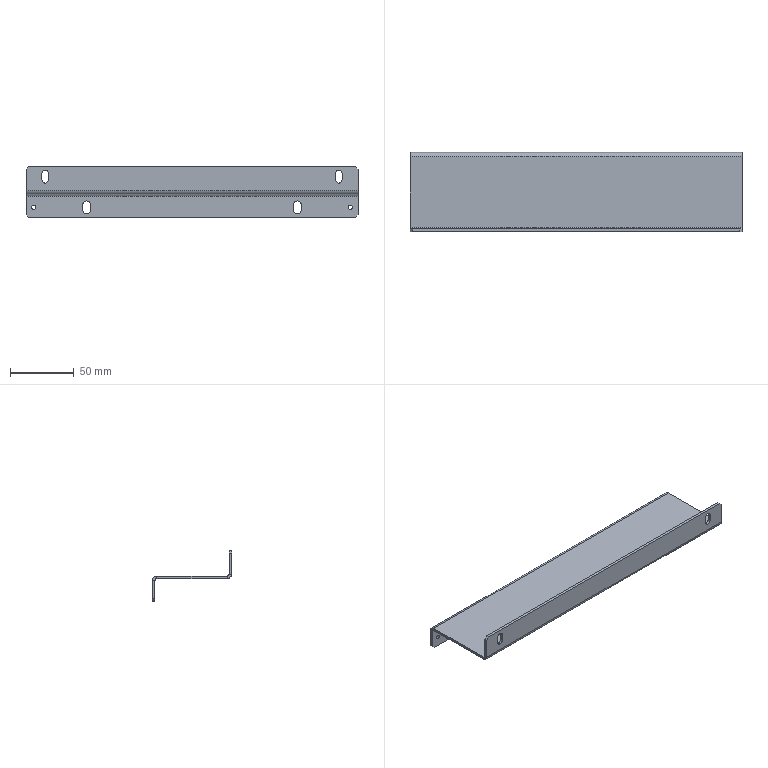Part | STEP file | 227H056377 Guide BKT_Default | 1 solid | 50 faces | box 260 x 62 x 40 mm | volume 50446 mm3 | plane 30 | cylinder 20 | commonest cylinder face diameters 5 x6 6 x6 3.3 x4 3 x2 7 x2